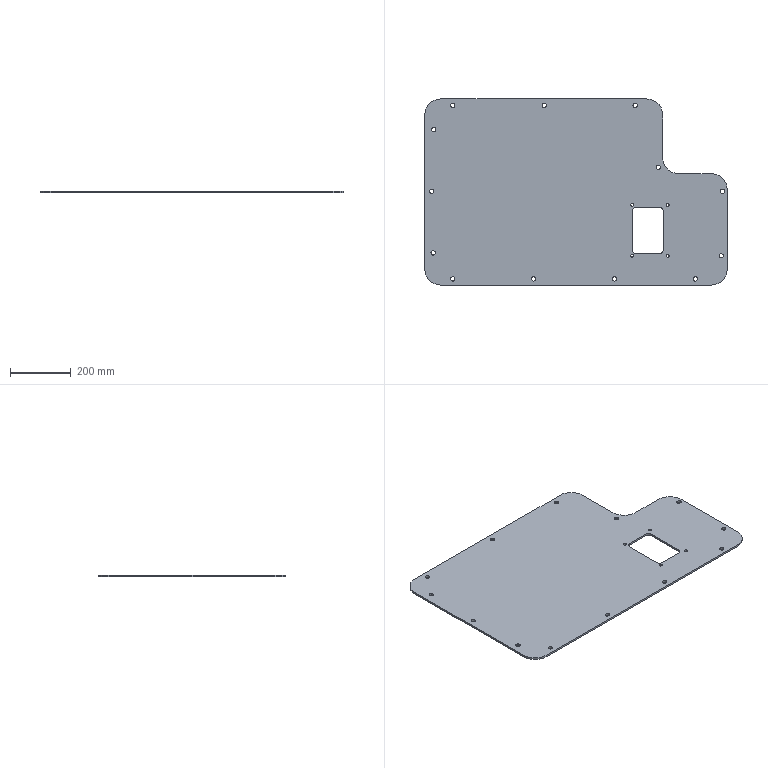Part | SolidWorks | features HoleWzd 2, Extrusion 1 | 1 solid | 56 faces | box 998 x 614.68 x 6.35 mm | volume 3433932 mm3 | cylinder 44 | plane 12 | commonest cylinder face diameters 14.288 x18 9.525 x8 14.287 x8 106.113 x6 25.4 x4